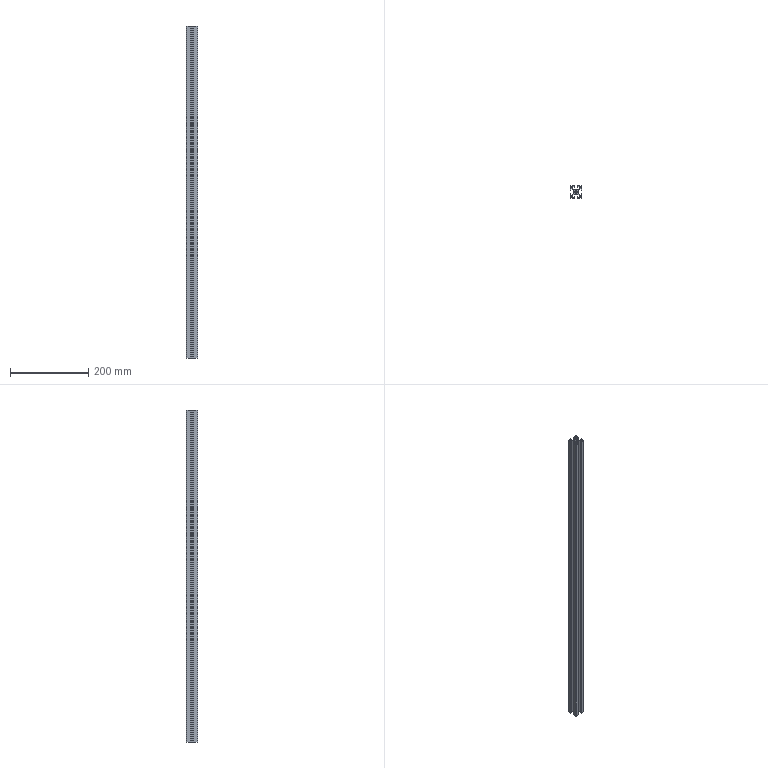Part | STEP file | SQ-8-3030W-850_Default | 1 solid | 84 faces | box 30 x 30 x 850 mm | volume 323559 mm3 | plane 62 | cylinder 22 | commonest cylinder face diameters 0.6 x8 4.2 x8 4 x4 6.8 x2